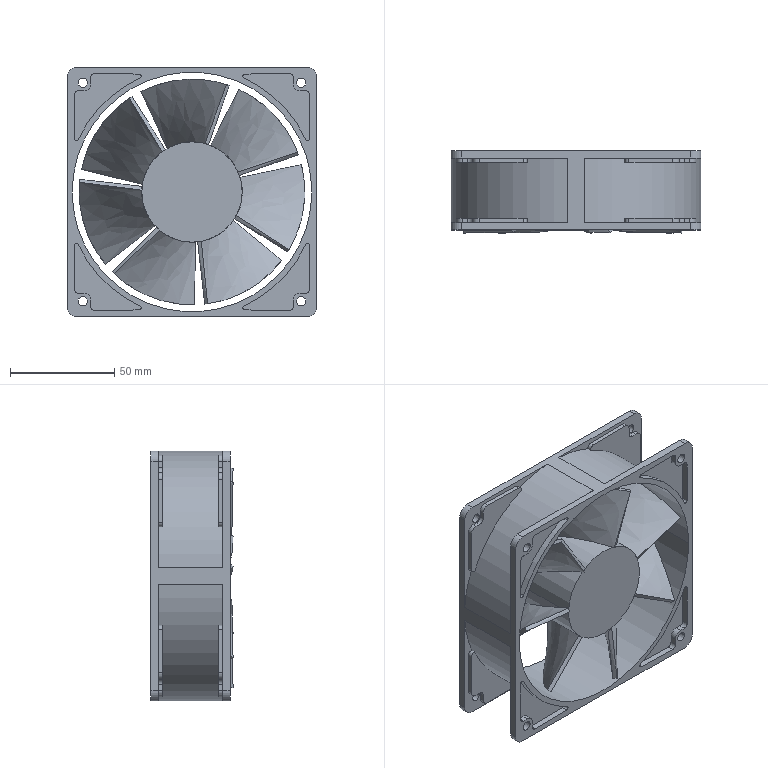Part | STEP file | Fan 9WV1224P1H00100 | 9 solids | 258 faces | box 120 x 39.419 x 120 mm | volume 145446 mm3 | cylinder 127 | plane 96 | spline 35 | commonest cylinder face diameters 4 x32 2 x16 4.5 x16 6 x16 120.247 x12 5 x8